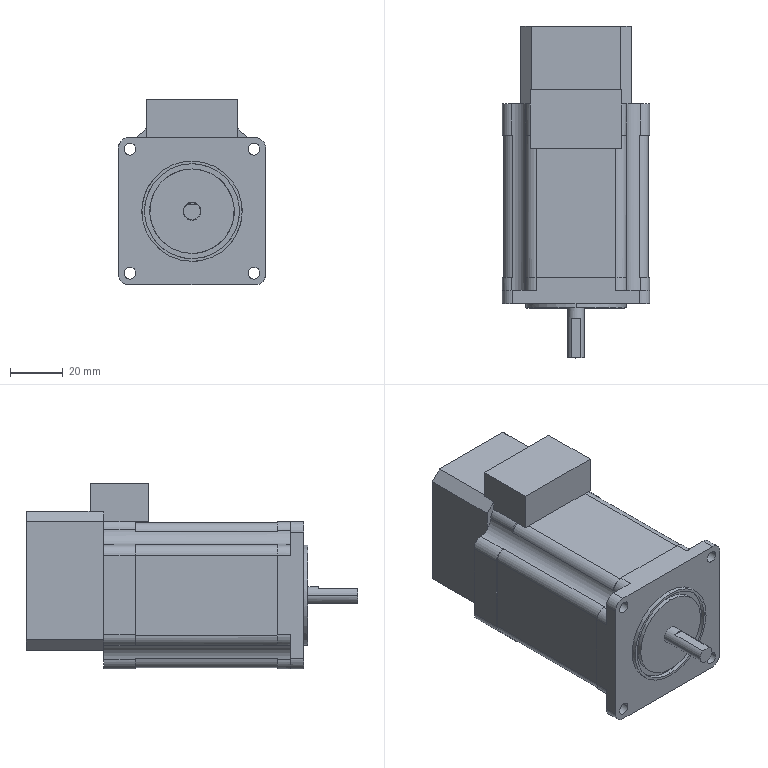Part | SolidWorks | features BaseBody 1 | 1 solid | 99 faces | box 56 x 126.1 x 70.6 mm | volume 288877 mm3 | cylinder 50 | plane 49 | commonest cylinder face diameters 8 x28 4.5 x8 12 x4 6.35 x2 6.85 x2 32.1 x2